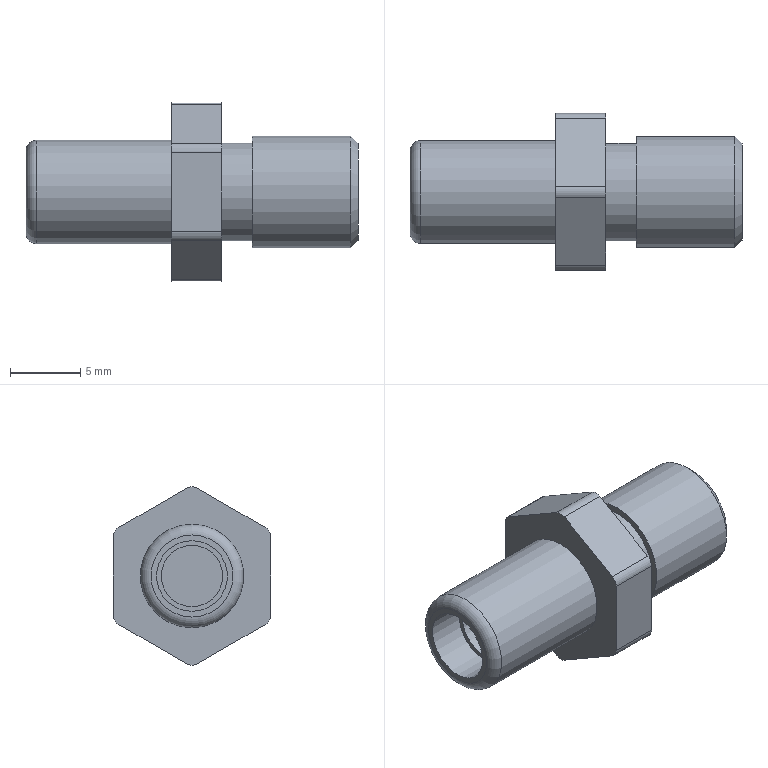Part | NX | features solid 2 | 1 solid | 28 faces | box 23.597 x 11.176 x 12.669 mm | volume 959.335 mm3 | plane 14 | cylinder 12 | torus 1 | cone 1 | commonest cylinder face diameters 1.524 x6 4.369 x2 5.029 x1 6.96 x1 7.366 x1 7.925 x1
STEP:
#1=CARTESIAN_POINT('',(0.,0.,2.184));
#2=VERTEX_POINT('',#1);
#3=CARTESIAN_POINT('',(0.,0.,0.));
#4=DIRECTION('',(-1.,0.,0.));
#5=DIRECTION('',(0.,0.,1.));
#6=AXIS2_PLACEMENT_3D('',#3,#4,#5);
#7=CIRCLE('',#6,2.184);
#8=EDGE_CURVE('',#2,#2,#7,.T.);
#9=ORIENTED_EDGE('',*,*,#8,.F.);
#10=EDGE_LOOP('',(#9));
#11=FACE_BOUND('',#10,.T.);
#12=CARTESIAN_POINT('',(-7.696,0.,-2.184));
#13=VERTEX_POINT('',#12);
#14=CARTESIAN_POINT('',(-7.696,0.,0.));
#15=DIRECTION('',(1.,0.,0.));
#16=DIRECTION('',(0.,0.,-1.));
#17=AXIS2_PLACEMENT_3D('',#14,#15,#16);
#18=CIRCLE('',#17,2.184);
#19=EDGE_CURVE('',#13,#13,#18,.T.);
#20=ORIENTED_EDGE('',*,*,#19,.F.);
#21=EDGE_LOOP('',(#20));
#22=FACE_BOUND('',#21,.T.);
#23=CARTESIAN_POINT('',(0.,0.,0.));
#24=DIRECTION('',(1.,0.,0.));
#25=DIRECTION('',(0.,0.,-1.));
#26=AXIS2_PLACEMENT_3D('',#23,#24,#25);
#27=CYLINDRICAL_SURFACE('',#26,2.184);
#28=ADVANCED_FACE('',(#11,#22),#27,.F.);
#29=CARTESIAN_POINT('',(0.,0.,-3.683));
#30=VERTEX_POINT('',#29);
#31=CARTESIAN_POINT('',(0.,0.,0.));
#32=DIRECTION('',(1.,0.,0.));
#33=DIRECTION('',(0.,0.,-1.));
#34=AXIS2_PLACEMENT_3D('',#31,#32,#33);
#35=CIRCLE('',#34,3.683);
#36=EDGE_CURVE('',#30,#30,#35,.T.);
#37=ORIENTED_EDGE('',*,*,#36,.T.);
#38=EDGE_LOOP('',(#37));
#39=FACE_BOUND('',#38,.T.);
#40=CARTESIAN_POINT('',(0.,5.207,3.446));
#41=VERTEX_POINT('',#40);
#42=CARTESIAN_POINT('',(0.,0.381,6.232));
#43=VERTEX_POINT('',#42);
#44=CARTESIAN_POINT('',(0.,5.588,3.226));
#45=DIRECTION('',(0.,-0.866,0.5));
#46=VECTOR('',#45,1000.);
#47=LINE('',#44,#46);
#48=EDGE_CURVE('',#41,#43,#47,.T.);
#49=ORIENTED_EDGE('',*,*,#48,.F.);
#50=CARTESIAN_POINT('',(0.,5.588,2.786));
#51=VERTEX_POINT('',#50);
#52=CARTESIAN_POINT('',(0.,4.826,2.786));
#53=DIRECTION('',(-1.,0.,0.));
#54=DIRECTION('',(0.,0.,1.));
#55=AXIS2_PLACEMENT_3D('',#52,#53,#54);
#56=CIRCLE('',#55,0.762);
#57=EDGE_CURVE('',#41,#51,#56,.T.);
#58=ORIENTED_EDGE('',*,*,#57,.T.);
#59=CARTESIAN_POINT('',(0.,5.588,-2.786));
#60=VERTEX_POINT('',#59);
#61=CARTESIAN_POINT('',(0.,5.588,-3.226));
#62=DIRECTION('',(0.,0.,1.));
#63=VECTOR('',#62,1000.);
#64=LINE('',#61,#63);
#65=EDGE_CURVE('',#60,#51,#64,.T.);
#66=ORIENTED_EDGE('',*,*,#65,.F.);
#67=CARTESIAN_POINT('',(0.,5.207,-3.446));
#68=VERTEX_POINT('',#67);
#69=CARTESIAN_POINT('',(0.,4.826,-2.786));
#70=DIRECTION('',(-1.,0.,0.));
#71=DIRECTION('',(0.,0.,1.));
#72=AXIS2_PLACEMENT_3D('',#69,#70,#71);
#73=CIRCLE('',#72,0.762);
#74=EDGE_CURVE('',#60,#68,#73,.T.);
#75=ORIENTED_EDGE('',*,*,#74,.T.);
#76=CARTESIAN_POINT('',(0.,0.381,-6.232));
#77=VERTEX_POINT('',#76);
#78=CARTESIAN_POINT('',(0.,0.,-6.452));
#79=DIRECTION('',(0.,0.866,0.5));
#80=VECTOR('',#79,1000.);
#81=LINE('',#78,#80);
#82=EDGE_CURVE('',#77,#68,#81,.T.);
#83=ORIENTED_EDGE('',*,*,#82,.F.);
#84=CARTESIAN_POINT('',(0.,-0.381,-6.232));
#85=VERTEX_POINT('',#84);
#86=CARTESIAN_POINT('',(0.,0.,-5.573));
#87=DIRECTION('',(-1.,0.,0.));
#88=DIRECTION('',(0.,0.,1.));
#89=AXIS2_PLACEMENT_3D('',#86,#87,#88);
#90=CIRCLE('',#89,0.762);
#91=EDGE_CURVE('',#77,#85,#90,.T.);
#92=ORIENTED_EDGE('',*,*,#91,.T.);
#93=CARTESIAN_POINT('',(0.,-5.207,-3.446));
#94=VERTEX_POINT('',#93);
#95=CARTESIAN_POINT('',(0.,-5.588,-3.226));
#96=DIRECTION('',(0.,0.866,-0.5));
#97=VECTOR('',#96,1000.);
#98=LINE('',#95,#97);
#99=EDGE_CURVE('',#94,#85,#98,.T.);
#100=ORIENTED_EDGE('',*,*,#99,.F.);
#101=CARTESIAN_POINT('',(0.,-5.588,-2.786));
#102=VERTEX_POINT('',#101);
#103=CARTESIAN_POINT('',(0.,-4.826,-2.786));
#104=DIRECTION('',(-1.,0.,0.));
#105=DIRECTION('',(0.,0.,1.));
#106=AXIS2_PLACEMENT_3D('',#103,#104,#105);
#107=CIRCLE('',#106,0.762);
#108=EDGE_CURVE('',#94,#102,#107,.T.);
#109=ORIENTED_EDGE('',*,*,#108,.T.);
#110=CARTESIAN_POINT('',(0.,-5.588,2.786));
#111=VERTEX_POINT('',#110);
#112=CARTESIAN_POINT('',(0.,-5.588,3.226));
#113=DIRECTION('',(0.,0.,-1.));
#114=VECTOR('',#113,1000.);
#115=LINE('',#112,#114);
#116=EDGE_CURVE('',#111,#102,#115,.T.);
#117=ORIENTED_EDGE('',*,*,#116,.F.);
#118=CARTESIAN_POINT('',(0.,-5.207,3.446));
#119=VERTEX_POINT('',#118);
#120=CARTESIAN_POINT('',(0.,-4.826,2.786));
#121=DIRECTION('',(-1.,0.,0.));
#122=DIRECTION('',(0.,0.,1.));
#123=AXIS2_PLACEMENT_3D('',#120,#121,#122);
#124=CIRCLE('',#123,0.762);
#125=EDGE_CURVE('',#111,#119,#124,.T.);
#126=ORIENTED_EDGE('',*,*,#125,.T.);
#127=CARTESIAN_POINT('',(0.,-0.381,6.232));
#128=VERTEX_POINT('',#127);
#129=CARTESIAN_POINT('',(0.,0.,6.452));
#130=DIRECTION('',(0.,-0.866,-0.5));
#131=VECTOR('',#130,1000.);
#132=LINE('',#129,#131);
#133=EDGE_CURVE('',#128,#119,#132,.T.);
#134=ORIENTED_EDGE('',*,*,#133,.F.);
#135=CARTESIAN_POINT('',(0.,0.,5.573));
#136=DIRECTION('',(-1.,0.,0.));
#137=DIRECTION('',(0.,0.,1.));
#138=AXIS2_PLACEMENT_3D('',#135,#136,#137);
#139=CIRCLE('',#138,0.762);
#140=EDGE_CURVE('',#128,#43,#139,.T.);
#141=ORIENTED_EDGE('',*,*,#140,.T.);
#142=EDGE_LOOP('',(#49,#58,#66,#75,#83,#92,#100,#109,#117,#126,#134,#141));
#143=FACE_BOUND('',#142,.T.);
#144=CARTESIAN_POINT('',(0.,3.683,0.));
#145=DIRECTION('',(-1.,0.,0.));
#146=DIRECTION('',(0.,0.,1.));
#147=AXIS2_PLACEMENT_3D('',#144,#145,#146);
#148=PLANE('',#147);
#149=ADVANCED_FACE('',(#39,#143),#148,.T.);
#150=CARTESIAN_POINT('',(-9.601,0.,3.683));
#151=VERTEX_POINT('',#150);
#152=CARTESIAN_POINT('',(-9.601,0.,0.));
#153=DIRECTION('',(-1.,0.,0.));
#154=DIRECTION('',(0.,0.,1.));
#155=AXIS2_PLACEMENT_3D('',#152,#153,#154);
#156=CIRCLE('',#155,3.683);
#157=EDGE_CURVE('',#151,#151,#156,.F.);
#158=ORIENTED_EDGE('',*,*,#157,.T.);
#159=EDGE_LOOP('',(#158));
#160=FACE_BOUND('',#159,.T.);
#161=ORIENTED_EDGE('',*,*,#36,.F.);
#162=EDGE_LOOP('',(#161));
#163=FACE_BOUND('',#162,.T.);
#164=CARTESIAN_POINT('',(0.,0.,0.));
#165=DIRECTION('',(1.,0.,0.));
#166=DIRECTION('',(0.,0.,-1.));
#167=AXIS2_PLACEMENT_3D('',#164,#165,#166);
#168=CYLINDRICAL_SURFACE('',#167,3.683);
#169=ADVANCED_FACE('',(#160,#163),#168,.T.);
#170=CARTESIAN_POINT('',(-10.363,0.,2.921));
#171=VERTEX_POINT('',#170);
#172=CARTESIAN_POINT('',(-10.363,0.,0.));
#173=DIRECTION('',(-1.,0.,0.));
#174=DIRECTION('',(0.,0.,1.));
#175=AXIS2_PLACEMENT_3D('',#172,#173,#174);
#176=CIRCLE('',#175,2.921);
#177=EDGE_CURVE('',#171,#171,#176,.T.);
#178=ORIENTED_EDGE('',*,*,#177,.T.);
#179=EDGE_LOOP('',(#178));
#180=FACE_BOUND('',#179,.T.);
#181=CARTESIAN_POINT('',(-10.363,0.,-2.515));
#182=VERTEX_POINT('',#181);
#183=CARTESIAN_POINT('',(-10.363,0.,0.));
#184=DIRECTION('',(1.,0.,0.));
#185=DIRECTION('',(0.,0.,-1.));
#186=AXIS2_PLACEMENT_3D('',#183,#184,#185);
#187=CIRCLE('',#186,2.515);
#188=EDGE_CURVE('',#182,#182,#187,.T.);
#189=ORIENTED_EDGE('',*,*,#188,.T.);
#190=EDGE_LOOP('',(#189));
#191=FACE_BOUND('',#190,.T.);
#192=CARTESIAN_POINT('',(-10.363,2.515,0.));
#193=DIRECTION('',(-1.,0.,0.));
#194=DIRECTION('',(0.,0.,1.));
#195=AXIS2_PLACEMENT_3D('',#192,#193,#194);
#196=PLANE('',#195);
#197=ADVANCED_FACE('',(#180,#191),#196,.T.);
#198=CARTESIAN_POINT('',(-7.696,0.,-2.515));
#199=VERTEX_POINT('',#198);
#200=CARTESIAN_POINT('',(-7.696,0.,0.));
#201=DIRECTION('',(1.,0.,0.));
#202=DIRECTION('',(0.,0.,-1.));
#203=AXIS2_PLACEMENT_3D('',#200,#201,#202);
#204=CIRCLE('',#203,2.515);
#205=EDGE_CURVE('',#199,#199,#204,.T.);
#206=ORIENTED_EDGE('',*,*,#205,.T.);
#207=EDGE_LOOP('',(#206));
#208=FACE_BOUND('',#207,.T.);
#209=ORIENTED_EDGE('',*,*,#188,.F.);
#210=EDGE_LOOP('',(#209));
#211=FACE_BOUND('',#210,.T.);
#212=CARTESIAN_POINT('',(0.,0.,0.));
#213=DIRECTION('',(1.,0.,0.));
#214=DIRECTION('',(0.,0.,-1.));
#215=AXIS2_PLACEMENT_3D('',#212,#213,#214);
#216=CYLINDRICAL_SURFACE('',#215,2.515);
#217=ADVANCED_FACE('',(#208,#211),#216,.F.);
#218=ORIENTED_EDGE('',*,*,#19,.T.);
#219=EDGE_LOOP('',(#218));
#220=FACE_BOUND('',#219,.T.);
#221=ORIENTED_EDGE('',*,*,#205,.F.);
#222=EDGE_LOOP('',(#221));
#223=FACE_BOUND('',#222,.T.);
#224=CARTESIAN_POINT('',(-7.696,2.515,0.));
#225=DIRECTION('',(-1.,0.,0.));
#226=DIRECTION('',(0.,0.,1.));
#227=AXIS2_PLACEMENT_3D('',#224,#225,#226);
#228=PLANE('',#227);
#229=ADVANCED_FACE('',(#220,#223),#228,.T.);
#230=ORIENTED_EDGE('',*,*,#177,.F.);
#231=EDGE_LOOP('',(#230));
#232=FACE_BOUND('',#231,.T.);
#233=ORIENTED_EDGE('',*,*,#157,.F.);
#234=EDGE_LOOP('',(#233));
#235=FACE_BOUND('',#234,.T.);
#236=CARTESIAN_POINT('',(-9.601,0.,0.));
#237=DIRECTION('',(-1.,0.,0.));
#238=DIRECTION('',(0.,0.,1.));
#239=AXIS2_PLACEMENT_3D('',#236,#237,#238);
#240=TOROIDAL_SURFACE('',#239,2.921,0.762);
#241=ADVANCED_FACE('',(#232,#235),#240,.T.);
#242=ORIENTED_EDGE('',*,*,#8,.T.);
#243=EDGE_LOOP('',(#242));
#244=FACE_BOUND('',#243,.T.);
#245=CARTESIAN_POINT('',(0.,5.588,-3.226));
#246=DIRECTION('',(-1.,0.,0.));
#247=DIRECTION('',(0.,0.,1.));
#248=AXIS2_PLACEMENT_3D('',#245,#246,#247);
#249=PLANE('',#248);
#250=ADVANCED_FACE('',(#244),#249,.T.);
#251=ORIENTED_EDGE('',*,*,#65,.T.);
#252=CARTESIAN_POINT('',(3.556,5.588,2.786));
#253=VERTEX_POINT('',#252);
#254=CARTESIAN_POINT('',(20.628,5.588,2.786));
#255=DIRECTION('',(-1.,0.,0.));
#256=VECTOR('',#255,1000.);
#257=LINE('',#254,#256);
#258=EDGE_CURVE('',#51,#253,#257,.F.);
#259=ORIENTED_EDGE('',*,*,#258,.T.);
#260=CARTESIAN_POINT('',(3.556,5.588,-2.786));
#261=VERTEX_POINT('',#260);
#262=CARTESIAN_POINT('',(3.556,5.588,-3.226));
#263=DIRECTION('',(0.,0.,1.));
#264=VECTOR('',#263,1000.);
#265=LINE('',#262,#264);
#266=EDGE_CURVE('',#261,#253,#265,.T.);
#267=ORIENTED_EDGE('',*,*,#266,.F.);
#268=CARTESIAN_POINT('',(20.628,5.588,-2.786));
#269=DIRECTION('',(-1.,0.,0.));
#270=VECTOR('',#269,1000.);
#271=LINE('',#268,#270);
#272=EDGE_CURVE('',#261,#60,#271,.T.);
#273=ORIENTED_EDGE('',*,*,#272,.T.);
#274=EDGE_LOOP('',(#251,#259,#267,#273));
#275=FACE_BOUND('',#274,.T.);
#276=CARTESIAN_POINT('',(20.628,5.588,-3.226));
#277=DIRECTION('',(0.,-1.,0.));
#278=DIRECTION('',(0.,0.,-1.));
#279=AXIS2_PLACEMENT_3D('',#276,#277,#278);
#280=PLANE('',#279);
#281=ADVANCED_FACE('',(#275),#280,.F.);
#282=CARTESIAN_POINT('',(3.556,5.207,3.446));
#283=VERTEX_POINT('',#282);
#284=CARTESIAN_POINT('',(3.556,0.381,6.232));
#285=VERTEX_POINT('',#284);
#286=CARTESIAN_POINT('',(3.556,5.588,3.226));
#287=DIRECTION('',(0.,-0.866,0.5));
#288=VECTOR('',#287,1000.);
#289=LINE('',#286,#288);
#290=EDGE_CURVE('',#283,#285,#289,.T.);
#291=ORIENTED_EDGE('',*,*,#290,.F.);
#292=CARTESIAN_POINT('',(20.628,5.207,3.446));
#293=DIRECTION('',(-1.,0.,0.));
#294=VECTOR('',#293,1000.);
#295=LINE('',#292,#294);
#296=EDGE_CURVE('',#283,#41,#295,.T.);
#297=ORIENTED_EDGE('',*,*,#296,.T.);
#298=ORIENTED_EDGE('',*,*,#48,.T.);
#299=CARTESIAN_POINT('',(20.628,0.381,6.232));
#300=DIRECTION('',(-1.,0.,0.));
#301=VECTOR('',#300,1000.);
#302=LINE('',#299,#301);
#303=EDGE_CURVE('',#43,#285,#302,.F.);
#304=ORIENTED_EDGE('',*,*,#303,.T.);
#305=EDGE_LOOP('',(#291,#297,#298,#304));
#306=FACE_BOUND('',#305,.T.);
#307=CARTESIAN_POINT('',(20.628,5.588,3.226));
#308=DIRECTION('',(0.,-0.5,-0.866));
#309=DIRECTION('',(0.,0.866,-0.5));
#310=AXIS2_PLACEMENT_3D('',#307,#308,#309);
#311=PLANE('',#310);
#312=ADVANCED_FACE('',(#306),#311,.F.);
#313=ORIENTED_EDGE('',*,*,#133,.T.);
#314=CARTESIAN_POINT('',(3.556,-5.207,3.446));
#315=VERTEX_POINT('',#314);
#316=CARTESIAN_POINT('',(20.628,-5.207,3.446));
#317=DIRECTION('',(-1.,0.,0.));
#318=VECTOR('',#317,1000.);
#319=LINE('',#316,#318);
#320=EDGE_CURVE('',#119,#315,#319,.F.);
#321=ORIENTED_EDGE('',*,*,#320,.T.);
#322=CARTESIAN_POINT('',(3.556,-0.381,6.232));
#323=VERTEX_POINT('',#322);
#324=CARTESIAN_POINT('',(3.556,0.,6.452));
#325=DIRECTION('',(0.,-0.866,-0.5));
#326=VECTOR('',#325,1000.);
#327=LINE('',#324,#326);
#328=EDGE_CURVE('',#323,#315,#327,.T.);
#329=ORIENTED_EDGE('',*,*,#328,.F.);
#330=CARTESIAN_POINT('',(20.628,-0.381,6.232));
#331=DIRECTION('',(-1.,0.,0.));
#332=VECTOR('',#331,1000.);
#333=LINE('',#330,#332);
#334=EDGE_CURVE('',#323,#128,#333,.T.);
#335=ORIENTED_EDGE('',*,*,#334,.T.);
#336=EDGE_LOOP('',(#313,#321,#329,#335));
#337=FACE_BOUND('',#336,.T.);
#338=CARTESIAN_POINT('',(20.628,0.,6.452));
#339=DIRECTION('',(0.,0.5,-0.866));
#340=DIRECTION('',(0.,0.866,0.5));
#341=AXIS2_PLACEMENT_3D('',#338,#339,#340);
#342=PLANE('',#341);
#343=ADVANCED_FACE('',(#337),#342,.F.);
#344=ORIENTED_EDGE('',*,*,#116,.T.);
#345=CARTESIAN_POINT('',(3.556,-5.588,-2.786));
#346=VERTEX_POINT('',#345);
#347=CARTESIAN_POINT('',(20.628,-5.588,-2.786));
#348=DIRECTION('',(-1.,0.,0.));
#349=VECTOR('',#348,1000.);
#350=LINE('',#347,#349);
#351=EDGE_CURVE('',#102,#346,#350,.F.);
#352=ORIENTED_EDGE('',*,*,#351,.T.);
#353=CARTESIAN_POINT('',(3.556,-5.588,2.786));
#354=VERTEX_POINT('',#353);
#355=CARTESIAN_POINT('',(3.556,-5.588,3.226));
#356=DIRECTION('',(0.,0.,-1.));
#357=VECTOR('',#356,1000.);
#358=LINE('',#355,#357);
#359=EDGE_CURVE('',#354,#346,#358,.T.);
#360=ORIENTED_EDGE('',*,*,#359,.F.);
#361=CARTESIAN_POINT('',(20.628,-5.588,2.786));
#362=DIRECTION('',(-1.,0.,0.));
#363=VECTOR('',#362,1000.);
#364=LINE('',#361,#363);
#365=EDGE_CURVE('',#354,#111,#364,.T.);
#366=ORIENTED_EDGE('',*,*,#365,.T.);
#367=EDGE_LOOP('',(#344,#352,#360,#366));
#368=FACE_BOUND('',#367,.T.);
#369=CARTESIAN_POINT('',(20.628,-5.588,3.226));
#370=DIRECTION('',(0.,1.,0.));
#371=DIRECTION('',(0.,0.,1.));
#372=AXIS2_PLACEMENT_3D('',#369,#370,#371);
#373=PLANE('',#372);
#374=ADVANCED_FACE('',(#368),#373,.F.);
#375=ORIENTED_EDGE('',*,*,#99,.T.);
#376=CARTESIAN_POINT('',(3.556,-0.381,-6.232));
#377=VERTEX_POINT('',#376);
#378=CARTESIAN_POINT('',(20.628,-0.381,-6.232));
#379=DIRECTION('',(-1.,0.,0.));
#380=VECTOR('',#379,1000.);
#381=LINE('',#378,#380);
#382=EDGE_CURVE('',#85,#377,#381,.F.);
#383=ORIENTED_EDGE('',*,*,#382,.T.);
#384=CARTESIAN_POINT('',(3.556,-5.207,-3.446));
#385=VERTEX_POINT('',#384);
#386=CARTESIAN_POINT('',(3.556,-5.588,-3.226));
#387=DIRECTION('',(0.,0.866,-0.5));
#388=VECTOR('',#387,1000.);
#389=LINE('',#386,#388);
#390=EDGE_CURVE('',#385,#377,#389,.T.);
#391=ORIENTED_EDGE('',*,*,#390,.F.);
#392=CARTESIAN_POINT('',(20.628,-5.207,-3.446));
#393=DIRECTION('',(-1.,0.,0.));
#394=VECTOR('',#393,1000.);
#395=LINE('',#392,#394);
#396=EDGE_CURVE('',#385,#94,#395,.T.);
#397=ORIENTED_EDGE('',*,*,#396,.T.);
#398=EDGE_LOOP('',(#375,#383,#391,#397));
#399=FACE_BOUND('',#398,.T.);
#400=CARTESIAN_POINT('',(20.628,-5.588,-3.226));
#401=DIRECTION('',(0.,0.5,0.866));
#402=DIRECTION('',(0.,-0.866,0.5));
#403=AXIS2_PLACEMENT_3D('',#400,#401,#402);
#404=PLANE('',#403);
#405=ADVANCED_FACE('',(#399),#404,.F.);
#406=ORIENTED_EDGE('',*,*,#82,.T.);
#407=CARTESIAN_POINT('',(3.556,5.207,-3.446));
#408=VERTEX_POINT('',#407);
#409=CARTESIAN_POINT('',(20.628,5.207,-3.446));
#410=DIRECTION('',(-1.,0.,0.));
#411=VECTOR('',#410,1000.);
#412=LINE('',#409,#411);
#413=EDGE_CURVE('',#68,#408,#412,.F.);
#414=ORIENTED_EDGE('',*,*,#413,.T.);
#415=CARTESIAN_POINT('',(3.556,0.381,-6.232));
#416=VERTEX_POINT('',#415);
#417=CARTESIAN_POINT('',(3.556,0.,-6.452));
#418=DIRECTION('',(0.,0.866,0.5));
#419=VECTOR('',#418,1000.);
#420=LINE('',#417,#419);
#421=EDGE_CURVE('',#416,#408,#420,.T.);
#422=ORIENTED_EDGE('',*,*,#421,.F.);
#423=CARTESIAN_POINT('',(20.628,0.381,-6.232));
#424=DIRECTION('',(-1.,0.,0.));
#425=VECTOR('',#424,1000.);
#426=LINE('',#423,#425);
#427=EDGE_CURVE('',#416,#77,#426,.T.);
#428=ORIENTED_EDGE('',*,*,#427,.T.);
#429=EDGE_LOOP('',(#406,#414,#422,#428));
#430=FACE_BOUND('',#429,.T.);
#431=CARTESIAN_POINT('',(20.628,0.,-6.452));
#432=DIRECTION('',(0.,-0.5,0.866));
#433=DIRECTION('',(0.,-0.866,-0.5));
#434=AXIS2_PLACEMENT_3D('',#431,#432,#433);
#435=PLANE('',#434);
#436=ADVANCED_FACE('',(#430),#435,.F.);
#437=CARTESIAN_POINT('',(5.715,0.,-3.48));
#438=VERTEX_POINT('',#437);
#439=CARTESIAN_POINT('',(5.715,0.,0.));
#440=DIRECTION('',(1.,0.,0.));
#441=DIRECTION('',(0.,0.,-1.));
#442=AXIS2_PLACEMENT_3D('',#439,#440,#441);
#443=CIRCLE('',#442,3.48);
#444=EDGE_CURVE('',#438,#438,#443,.T.);
#445=ORIENTED_EDGE('',*,*,#444,.T.);
#446=EDGE_LOOP('',(#445));
#447=FACE_BOUND('',#446,.T.);
#448=CARTESIAN_POINT('',(5.715,0.,-3.962));
#449=VERTEX_POINT('',#448);
#450=CARTESIAN_POINT('',(5.715,0.,0.));
#451=DIRECTION('',(1.,0.,0.));
#452=DIRECTION('',(0.,0.,-1.));
#453=AXIS2_PLACEMENT_3D('',#450,#451,#452);
#454=CIRCLE('',#453,3.962);
#455=EDGE_CURVE('',#449,#449,#454,.T.);
#456=ORIENTED_EDGE('',*,*,#455,.F.);
#457=EDGE_LOOP('',(#456));
#458=FACE_BOUND('',#457,.T.);
#459=CARTESIAN_POINT('',(5.715,3.962,0.));
#460=DIRECTION('',(-1.,0.,0.));
#461=DIRECTION('',(0.,0.,1.));
#462=AXIS2_PLACEMENT_3D('',#459,#460,#461);
#463=PLANE('',#462);
#464=ADVANCED_FACE('',(#447,#458),#463,.T.);
#465=CARTESIAN_POINT('',(3.556,0.,-3.48));
#466=VERTEX_POINT('',#465);
#467=CARTESIAN_POINT('',(3.556,0.,0.));
#468=DIRECTION('',(1.,0.,0.));
#469=DIRECTION('',(0.,0.,-1.));
#470=AXIS2_PLACEMENT_3D('',#467,#468,#469);
#471=CIRCLE('',#470,3.48);
#472=EDGE_CURVE('',#466,#466,#471,.T.);
#473=ORIENTED_EDGE('',*,*,#472,.T.);
#474=EDGE_LOOP('',(#473));
#475=FACE_BOUND('',#474,.T.);
#476=ORIENTED_EDGE('',*,*,#444,.F.);
#477=EDGE_LOOP('',(#476));
#478=FACE_BOUND('',#477,.T.);
#479=CARTESIAN_POINT('',(0.,0.,0.));
#480=DIRECTION('',(1.,0.,0.));
#481=DIRECTION('',(0.,0.,-1.));
#482=AXIS2_PLACEMENT_3D('',#479,#480,#481);
#483=CYLINDRICAL_SURFACE('',#482,3.48);
#484=ADVANCED_FACE('',(#475,#478),#483,.T.);
#485=ORIENTED_EDGE('',*,*,#266,.T.);
#486=CARTESIAN_POINT('',(3.556,4.826,2.786));
#487=DIRECTION('',(1.,0.,0.));
#488=DIRECTION('',(0.,0.,-1.));
#489=AXIS2_PLACEMENT_3D('',#486,#487,#488);
#490=CIRCLE('',#489,0.762);
#491=EDGE_CURVE('',#253,#283,#490,.T.);
#492=ORIENTED_EDGE('',*,*,#491,.T.);
#493=ORIENTED_EDGE('',*,*,#290,.T.);
#494=CARTESIAN_POINT('',(3.556,0.,5.573));
#495=DIRECTION('',(1.,0.,0.));
#496=DIRECTION('',(0.,0.,-1.));
#497=AXIS2_PLACEMENT_3D('',#494,#495,#496);
#498=CIRCLE('',#497,0.762);
#499=EDGE_CURVE('',#285,#323,#498,.T.);
#500=ORIENTED_EDGE('',*,*,#499,.T.);
#501=ORIENTED_EDGE('',*,*,#328,.T.);
#502=CARTESIAN_POINT('',(3.556,-4.826,2.786));
#503=DIRECTION('',(1.,0.,0.));
#504=DIRECTION('',(0.,0.,-1.));
#505=AXIS2_PLACEMENT_3D('',#502,#503,#504);
#506=CIRCLE('',#505,0.762);
#507=EDGE_CURVE('',#315,#354,#506,.T.);
#508=ORIENTED_EDGE('',*,*,#507,.T.);
#509=ORIENTED_EDGE('',*,*,#359,.T.);
#510=CARTESIAN_POINT('',(3.556,-4.826,-2.786));
#511=DIRECTION('',(1.,0.,0.));
#512=DIRECTION('',(0.,0.,-1.));
#513=AXIS2_PLACEMENT_3D('',#510,#511,#512);
#514=CIRCLE('',#513,0.762);
#515=EDGE_CURVE('',#346,#385,#514,.T.);
#516=ORIENTED_EDGE('',*,*,#515,.T.);
#517=ORIENTED_EDGE('',*,*,#390,.T.);
#518=CARTESIAN_POINT('',(3.556,0.,-5.573));
#519=DIRECTION('',(1.,0.,0.));
#520=DIRECTION('',(0.,0.,-1.));
#521=AXIS2_PLACEMENT_3D('',#518,#519,#520);
#522=CIRCLE('',#521,0.762);
#523=EDGE_CURVE('',#377,#416,#522,.T.);
#524=ORIENTED_EDGE('',*,*,#523,.T.);
#525=ORIENTED_EDGE('',*,*,#421,.T.);
#526=CARTESIAN_POINT('',(3.556,4.826,-2.786));
#527=DIRECTION('',(1.,0.,0.));
#528=DIRECTION('',(0.,0.,-1.));
#529=AXIS2_PLACEMENT_3D('',#526,#527,#528);
#530=CIRCLE('',#529,0.762);
#531=EDGE_CURVE('',#408,#261,#530,.T.);
#532=ORIENTED_EDGE('',*,*,#531,.T.);
#533=EDGE_LOOP('',(#485,#492,#493,#500,#501,#508,#509,#516,#517,#524,#525,#532));
#534=FACE_BOUND('',#533,.T.);
#535=ORIENTED_EDGE('',*,*,#472,.F.);
#536=EDGE_LOOP('',(#535));
#537=FACE_BOUND('',#536,.T.);
#538=CARTESIAN_POINT('',(3.556,5.588,0.));
#539=DIRECTION('',(1.,0.,0.));
#540=DIRECTION('',(0.,0.,-1.));
#541=AXIS2_PLACEMENT_3D('',#538,#539,#540);
#542=PLANE('',#541);
#543=ADVANCED_FACE('',(#534,#537),#542,.T.);
#544=CARTESIAN_POINT('',(12.725,0.,-3.962));
#545=VERTEX_POINT('',#544);
#546=CARTESIAN_POINT('',(12.725,0.,0.));
#547=DIRECTION('',(1.,0.,0.));
#548=DIRECTION('',(0.,0.,-1.));
#549=AXIS2_PLACEMENT_3D('',#546,#547,#548);
#550=CIRCLE('',#549,3.962);
#551=EDGE_CURVE('',#545,#545,#550,.F.);
#552=ORIENTED_EDGE('',*,*,#551,.T.);
#553=EDGE_LOOP('',(#552));
#554=FACE_BOUND('',#553,.T.);
#555=ORIENTED_EDGE('',*,*,#455,.T.);
#556=EDGE_LOOP('',(#555));
#557=FACE_BOUND('',#556,.T.);
#558=CARTESIAN_POINT('',(0.,0.,0.));
#559=DIRECTION('',(1.,0.,0.));
#560=DIRECTION('',(0.,0.,-1.));
#561=AXIS2_PLACEMENT_3D('',#558,#559,#560);
#562=CYLINDRICAL_SURFACE('',#561,3.962);
#563=ADVANCED_FACE('',(#554,#557),#562,.T.);
#564=ORIENTED_EDGE('',*,*,#551,.F.);
#565=EDGE_LOOP('',(#564));
#566=FACE_BOUND('',#565,.T.);
#567=CARTESIAN_POINT('',(13.233,0.,-3.454));
#568=VERTEX_POINT('',#567);
#569=CARTESIAN_POINT('',(13.233,0.,0.));
#570=DIRECTION('',(1.,0.,0.));
#571=DIRECTION('',(0.,0.,-1.));
#572=AXIS2_PLACEMENT_3D('',#569,#570,#571);
#573=CIRCLE('',#572,3.454);
#574=EDGE_CURVE('',#568,#568,#573,.T.);
#575=ORIENTED_EDGE('',*,*,#574,.F.);
#576=EDGE_LOOP('',(#575));
#577=FACE_BOUND('',#576,.T.);
#578=CARTESIAN_POINT('',(13.233,0.,0.));
#579=DIRECTION('',(-1.,0.,0.));
#580=DIRECTION('',(0.,0.,1.));
#581=AXIS2_PLACEMENT_3D('',#578,#579,#580);
#582=CONICAL_SURFACE('',#581,3.454,0.7854);
#583=ADVANCED_FACE('',(#566,#577),#582,.T.);
#584=ORIENTED_EDGE('',*,*,#574,.T.);
#585=EDGE_LOOP('',(#584));
#586=FACE_BOUND('',#585,.T.);
#587=CARTESIAN_POINT('',(13.233,0.,-2.184));
#588=VERTEX_POINT('',#587);
#589=CARTESIAN_POINT('',(13.233,0.,0.));
#590=DIRECTION('',(1.,0.,0.));
#591=DIRECTION('',(0.,0.,-1.));
#592=AXIS2_PLACEMENT_3D('',#589,#590,#591);
#593=CIRCLE('',#592,2.184);
#594=EDGE_CURVE('',#588,#588,#593,.T.);
#595=ORIENTED_EDGE('',*,*,#594,.F.);
#596=EDGE_LOOP('',(#595));
#597=FACE_BOUND('',#596,.T.);
#598=CARTESIAN_POINT('',(13.233,2.184,0.));
#599=DIRECTION('',(1.,0.,0.));
#600=DIRECTION('',(0.,0.,-1.));
#601=AXIS2_PLACEMENT_3D('',#598,#599,#600);
#602=PLANE('',#601);
#603=ADVANCED_FACE('',(#586,#597),#602,.T.);
#604=CARTESIAN_POINT('',(3.556,0.,-2.184));
#605=VERTEX_POINT('',#604);
#606=CARTESIAN_POINT('',(3.556,0.,0.));
#607=DIRECTION('',(1.,0.,0.));
#608=DIRECTION('',(0.,0.,-1.));
#609=AXIS2_PLACEMENT_3D('',#606,#607,#608);
#610=CIRCLE('',#609,2.184);
#611=EDGE_CURVE('',#605,#605,#610,.T.);
#612=ORIENTED_EDGE('',*,*,#611,.F.);
#613=EDGE_LOOP('',(#612));
#614=FACE_BOUND('',#613,.T.);
#615=ORIENTED_EDGE('',*,*,#594,.T.);
#616=EDGE_LOOP('',(#615));
#617=FACE_BOUND('',#616,.T.);
#618=CARTESIAN_POINT('',(0.,0.,0.));
#619=DIRECTION('',(1.,0.,0.));
#620=DIRECTION('',(0.,0.,-1.));
#621=AXIS2_PLACEMENT_3D('',#618,#619,#620);
#622=CYLINDRICAL_SURFACE('',#621,2.184);
#623=ADVANCED_FACE('',(#614,#617),#622,.F.);
#624=ORIENTED_EDGE('',*,*,#611,.T.);
#625=EDGE_LOOP('',(#624));
#626=FACE_BOUND('',#625,.T.);
#627=CARTESIAN_POINT('',(3.556,5.588,0.));
#628=DIRECTION('',(1.,0.,0.));
#629=DIRECTION('',(0.,0.,-1.));
#630=AXIS2_PLACEMENT_3D('',#627,#628,#629);
#631=PLANE('',#630);
#632=ADVANCED_FACE('',(#626),#631,.T.);
#633=ORIENTED_EDGE('',*,*,#491,.F.);
#634=ORIENTED_EDGE('',*,*,#258,.F.);
#635=ORIENTED_EDGE('',*,*,#57,.F.);
#636=ORIENTED_EDGE('',*,*,#296,.F.);
#637=EDGE_LOOP('',(#633,#634,#635,#636));
#638=FACE_BOUND('',#637,.T.);
#639=CARTESIAN_POINT('',(20.628,4.826,2.786));
#640=DIRECTION('',(-1.,0.,0.));
#641=DIRECTION('',(0.,0.,1.));
#642=AXIS2_PLACEMENT_3D('',#639,#640,#641);
#643=CYLINDRICAL_SURFACE('',#642,0.762);
#644=ADVANCED_FACE('',(#638),#643,.T.);
#645=ORIENTED_EDGE('',*,*,#531,.F.);
#646=ORIENTED_EDGE('',*,*,#413,.F.);
#647=ORIENTED_EDGE('',*,*,#74,.F.);
#648=ORIENTED_EDGE('',*,*,#272,.F.);
#649=EDGE_LOOP('',(#645,#646,#647,#648));
#650=FACE_BOUND('',#649,.T.);
#651=CARTESIAN_POINT('',(20.628,4.826,-2.786));
#652=DIRECTION('',(-1.,0.,0.));
#653=DIRECTION('',(0.,0.,1.));
#654=AXIS2_PLACEMENT_3D('',#651,#652,#653);
#655=CYLINDRICAL_SURFACE('',#654,0.762);
#656=ADVANCED_FACE('',(#650),#655,.T.);
#657=ORIENTED_EDGE('',*,*,#523,.F.);
#658=ORIENTED_EDGE('',*,*,#382,.F.);
#659=ORIENTED_EDGE('',*,*,#91,.F.);
#660=ORIENTED_EDGE('',*,*,#427,.F.);
#661=EDGE_LOOP('',(#657,#658,#659,#660));
#662=FACE_BOUND('',#661,.T.);
#663=CARTESIAN_POINT('',(20.628,0.,-5.573));
#664=DIRECTION('',(-1.,0.,0.));
#665=DIRECTION('',(0.,0.,1.));
#666=AXIS2_PLACEMENT_3D('',#663,#664,#665);
#667=CYLINDRICAL_SURFACE('',#666,0.762);
#668=ADVANCED_FACE('',(#662),#667,.T.);
#669=ORIENTED_EDGE('',*,*,#515,.F.);
#670=ORIENTED_EDGE('',*,*,#351,.F.);
#671=ORIENTED_EDGE('',*,*,#108,.F.);
#672=ORIENTED_EDGE('',*,*,#396,.F.);
#673=EDGE_LOOP('',(#669,#670,#671,#672));
#674=FACE_BOUND('',#673,.T.);
#675=CARTESIAN_POINT('',(20.628,-4.826,-2.786));
#676=DIRECTION('',(-1.,0.,0.));
#677=DIRECTION('',(0.,0.,1.));
#678=AXIS2_PLACEMENT_3D('',#675,#676,#677);
#679=CYLINDRICAL_SURFACE('',#678,0.762);
#680=ADVANCED_FACE('',(#674),#679,.T.);
#681=ORIENTED_EDGE('',*,*,#507,.F.);
#682=ORIENTED_EDGE('',*,*,#320,.F.);
#683=ORIENTED_EDGE('',*,*,#125,.F.);
#684=ORIENTED_EDGE('',*,*,#365,.F.);
#685=EDGE_LOOP('',(#681,#682,#683,#684));
#686=FACE_BOUND('',#685,.T.);
#687=CARTESIAN_POINT('',(20.628,-4.826,2.786));
#688=DIRECTION('',(-1.,0.,0.));
#689=DIRECTION('',(0.,0.,1.));
#690=AXIS2_PLACEMENT_3D('',#687,#688,#689);
#691=CYLINDRICAL_SURFACE('',#690,0.762);
#692=ADVANCED_FACE('',(#686),#691,.T.);
#693=ORIENTED_EDGE('',*,*,#499,.F.);
#694=ORIENTED_EDGE('',*,*,#303,.F.);
#695=ORIENTED_EDGE('',*,*,#140,.F.);
#696=ORIENTED_EDGE('',*,*,#334,.F.);
#697=EDGE_LOOP('',(#693,#694,#695,#696));
#698=FACE_BOUND('',#697,.T.);
#699=CARTESIAN_POINT('',(20.628,0.,5.573));
#700=DIRECTION('',(-1.,0.,0.));
#701=DIRECTION('',(0.,0.,1.));
#702=AXIS2_PLACEMENT_3D('',#699,#700,#701);
#703=CYLINDRICAL_SURFACE('',#702,0.762);
#704=ADVANCED_FACE('',(#698),#703,.T.);
#705=CLOSED_SHELL('',(#28,#149,#169,#197,#217,#229,#241,#250,#281,#312,#343,#374,#405,#436,#464,#484,#543,#563,#583,#603,#623,#632,#644,#656,#668,#680,#692,#704));
#706=MANIFOLD_SOLID_BREP('',#705);
#707=(LENGTH_UNIT()NAMED_UNIT(*)SI_UNIT(.MILLI.,.METRE.));
#708=UNCERTAINTY_MEASURE_WITH_UNIT(LENGTH_MEASURE(0.00001),#707,'','');
#709=(NAMED_UNIT(*)PLANE_ANGLE_UNIT()SI_UNIT($,.RADIAN.));
#710=(NAMED_UNIT(*)SI_UNIT($,.STERADIAN.)SOLID_ANGLE_UNIT());
#711=(GEOMETRIC_REPRESENTATION_CONTEXT(3)GLOBAL_UNCERTAINTY_ASSIGNED_CONTEXT((#708))GLOBAL_UNIT_ASSIGNED_CONTEXT((#707,#709,#710))REPRESENTATION_CONTEXT('',''));
#712=ADVANCED_BREP_SHAPE_REPRESENTATION('',(#706),#711);